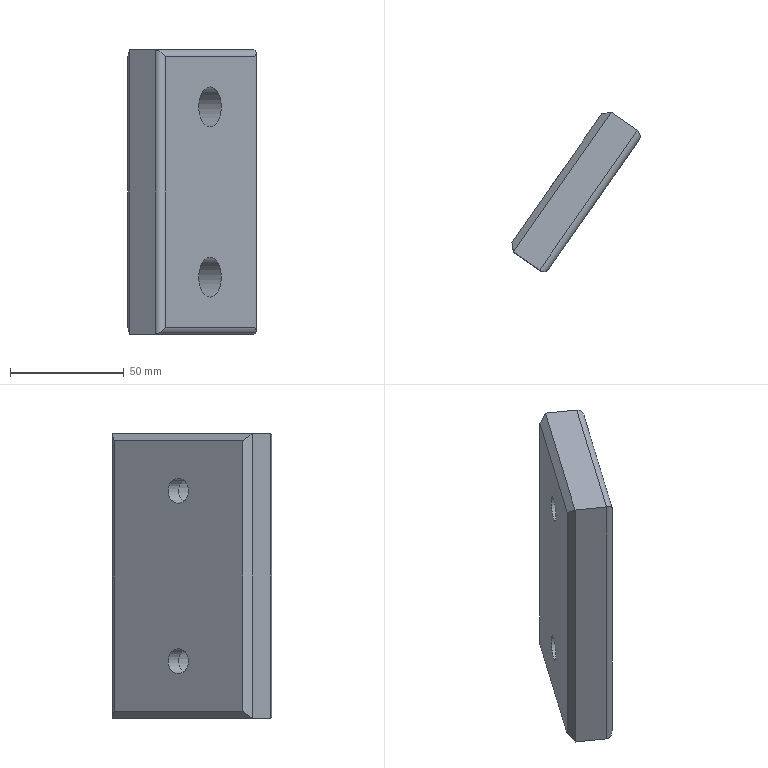Part | NX | features solid 2 | 1 solid | 20 faces | box 56.502 x 70.009 x 125 mm | volume 177681 mm3 | plane 12 | cylinder 8 | commonest cylinder face diameters 6 x4 11 x2 17.5 x2
STEP:
#1=CARTESIAN_POINT('',(279.908,328.94,26.883));
#2=VERTEX_POINT('',#1);
#3=CARTESIAN_POINT('',(291.376,320.91,26.883));
#4=VERTEX_POINT('',#3);
#5=CARTESIAN_POINT('',(277.45,330.66,26.883));
#6=DIRECTION('',(0.8192,-0.5736,0.));
#7=VECTOR('',#6,1000.);
#8=LINE('',#5,#7);
#9=EDGE_CURVE('',#2,#4,#8,.T.);
#10=ORIENTED_EDGE('',*,*,#9,.F.);
#11=CARTESIAN_POINT('',(236.889,267.503,26.883));
#12=VERTEX_POINT('',#11);
#13=CARTESIAN_POINT('',(236.889,267.503,26.883));
#14=DIRECTION('',(-0.5736,-0.8192,0.));
#15=VECTOR('',#14,1000.);
#16=LINE('',#13,#15);
#17=EDGE_CURVE('',#2,#12,#16,.T.);
#18=ORIENTED_EDGE('',*,*,#17,.T.);
#19=CARTESIAN_POINT('',(248.357,259.473,26.883));
#20=VERTEX_POINT('',#19);
#21=CARTESIAN_POINT('',(234.432,269.224,26.883));
#22=DIRECTION('',(0.8192,-0.5736,0.));
#23=VECTOR('',#22,1000.);
#24=LINE('',#21,#23);
#25=EDGE_CURVE('',#12,#20,#24,.T.);
#26=ORIENTED_EDGE('',*,*,#25,.T.);
#27=CARTESIAN_POINT('',(248.357,259.473,26.883));
#28=DIRECTION('',(0.5736,0.8192,0.));
#29=VECTOR('',#28,1000.);
#30=LINE('',#27,#29);
#31=EDGE_CURVE('',#20,#4,#30,.T.);
#32=ORIENTED_EDGE('',*,*,#31,.T.);
#33=EDGE_LOOP('',(#10,#18,#26,#32));
#34=FACE_BOUND('',#33,.T.);
#35=CARTESIAN_POINT('',(234.432,269.224,26.883));
#36=DIRECTION('',(0.,0.,-1.));
#37=DIRECTION('',(0.8192,-0.5736,0.));
#38=AXIS2_PLACEMENT_3D('',#35,#36,#37);
#39=PLANE('',#38);
#40=ADVANCED_FACE('',(#34),#39,.F.);
#41=CARTESIAN_POINT('',(279.908,328.94,-98.117));
#42=VERTEX_POINT('',#41);
#43=CARTESIAN_POINT('',(291.376,320.91,-98.117));
#44=VERTEX_POINT('',#43);
#45=CARTESIAN_POINT('',(277.45,330.66,-98.117));
#46=DIRECTION('',(0.8192,-0.5736,0.));
#47=VECTOR('',#46,1000.);
#48=LINE('',#45,#47);
#49=EDGE_CURVE('',#42,#44,#48,.T.);
#50=ORIENTED_EDGE('',*,*,#49,.F.);
#51=CARTESIAN_POINT('',(279.908,328.94,26.883));
#52=DIRECTION('',(0.,0.,1.));
#53=VECTOR('',#52,1000.);
#54=LINE('',#51,#53);
#55=EDGE_CURVE('',#42,#2,#54,.T.);
#56=ORIENTED_EDGE('',*,*,#55,.T.);
#57=ORIENTED_EDGE('',*,*,#9,.T.);
#58=CARTESIAN_POINT('',(291.376,320.91,26.883));
#59=DIRECTION('',(0.,0.,-1.));
#60=VECTOR('',#59,1000.);
#61=LINE('',#58,#60);
#62=EDGE_CURVE('',#4,#44,#61,.T.);
#63=ORIENTED_EDGE('',*,*,#62,.T.);
#64=EDGE_LOOP('',(#50,#56,#57,#63));
#65=FACE_BOUND('',#64,.T.);
#66=CARTESIAN_POINT('',(277.45,330.66,26.883));
#67=DIRECTION('',(-0.5736,-0.8192,0.));
#68=DIRECTION('',(-0.8192,0.5736,0.));
#69=AXIS2_PLACEMENT_3D('',#66,#67,#68);
#70=PLANE('',#69);
#71=ADVANCED_FACE('',(#65),#70,.F.);
#72=CARTESIAN_POINT('',(236.889,267.503,-98.117));
#73=VERTEX_POINT('',#72);
#74=CARTESIAN_POINT('',(248.357,259.473,-98.117));
#75=VERTEX_POINT('',#74);
#76=CARTESIAN_POINT('',(234.432,269.224,-98.117));
#77=DIRECTION('',(0.8192,-0.5736,0.));
#78=VECTOR('',#77,1000.);
#79=LINE('',#76,#78);
#80=EDGE_CURVE('',#73,#75,#79,.T.);
#81=ORIENTED_EDGE('',*,*,#80,.F.);
#82=CARTESIAN_POINT('',(279.908,328.94,-98.117));
#83=DIRECTION('',(0.5736,0.8192,0.));
#84=VECTOR('',#83,1000.);
#85=LINE('',#82,#84);
#86=EDGE_CURVE('',#73,#42,#85,.T.);
#87=ORIENTED_EDGE('',*,*,#86,.T.);
#88=ORIENTED_EDGE('',*,*,#49,.T.);
#89=CARTESIAN_POINT('',(291.376,320.91,-98.117));
#90=DIRECTION('',(-0.5736,-0.8192,0.));
#91=VECTOR('',#90,1000.);
#92=LINE('',#89,#91);
#93=EDGE_CURVE('',#44,#75,#92,.T.);
#94=ORIENTED_EDGE('',*,*,#93,.T.);
#95=EDGE_LOOP('',(#81,#87,#88,#94));
#96=FACE_BOUND('',#95,.T.);
#97=CARTESIAN_POINT('',(277.45,330.66,-98.117));
#98=DIRECTION('',(0.,0.,1.));
#99=DIRECTION('',(-0.8192,0.5736,0.));
#100=AXIS2_PLACEMENT_3D('',#97,#98,#99);
#101=PLANE('',#100);
#102=ADVANCED_FACE('',(#96),#101,.F.);
#103=ORIENTED_EDGE('',*,*,#25,.F.);
#104=CARTESIAN_POINT('',(236.889,267.503,-173.117));
#105=DIRECTION('',(0.,0.,-1.));
#106=VECTOR('',#105,1000.);
#107=LINE('',#104,#106);
#108=EDGE_CURVE('',#12,#73,#107,.T.);
#109=ORIENTED_EDGE('',*,*,#108,.T.);
#110=ORIENTED_EDGE('',*,*,#80,.T.);
#111=CARTESIAN_POINT('',(248.357,259.473,-173.117));
#112=DIRECTION('',(0.,0.,1.));
#113=VECTOR('',#112,1000.);
#114=LINE('',#111,#113);
#115=EDGE_CURVE('',#75,#20,#114,.T.);
#116=ORIENTED_EDGE('',*,*,#115,.T.);
#117=EDGE_LOOP('',(#103,#109,#110,#116));
#118=FACE_BOUND('',#117,.T.);
#119=CARTESIAN_POINT('',(234.432,269.224,-173.117));
#120=DIRECTION('',(0.5736,0.8192,0.));
#121=DIRECTION('',(0.,0.,-1.));
#122=AXIS2_PLACEMENT_3D('',#119,#120,#121);
#123=PLANE('',#122);
#124=ADVANCED_FACE('',(#118),#123,.F.);
#125=CARTESIAN_POINT('',(275.729,328.203,23.883));
#126=VERTEX_POINT('',#125);
#127=CARTESIAN_POINT('',(275.729,328.203,-95.117));
#128=VERTEX_POINT('',#127);
#129=CARTESIAN_POINT('',(275.729,328.203,-173.117));
#130=DIRECTION('',(0.,0.,-1.));
#131=VECTOR('',#130,1000.);
#132=LINE('',#129,#131);
#133=EDGE_CURVE('',#126,#128,#132,.T.);
#134=ORIENTED_EDGE('',*,*,#133,.T.);
#135=CARTESIAN_POINT('',(236.153,271.681,-95.117));
#136=VERTEX_POINT('',#135);
#137=CARTESIAN_POINT('',(234.432,269.224,-95.117));
#138=DIRECTION('',(-0.5736,-0.8192,0.));
#139=VECTOR('',#138,1000.);
#140=LINE('',#137,#139);
#141=EDGE_CURVE('',#128,#136,#140,.T.);
#142=ORIENTED_EDGE('',*,*,#141,.T.);
#143=CARTESIAN_POINT('',(236.153,271.681,23.883));
#144=VERTEX_POINT('',#143);
#145=CARTESIAN_POINT('',(236.153,271.681,26.883));
#146=DIRECTION('',(0.,0.,1.));
#147=VECTOR('',#146,1000.);
#148=LINE('',#145,#147);
#149=EDGE_CURVE('',#136,#144,#148,.T.);
#150=ORIENTED_EDGE('',*,*,#149,.T.);
#151=CARTESIAN_POINT('',(277.45,330.66,23.883));
#152=DIRECTION('',(0.5736,0.8192,0.));
#153=VECTOR('',#152,1000.);
#154=LINE('',#151,#153);
#155=EDGE_CURVE('',#144,#126,#154,.T.);
#156=ORIENTED_EDGE('',*,*,#155,.T.);
#157=EDGE_LOOP('',(#134,#142,#150,#156));
#158=FACE_BOUND('',#157,.T.);
#159=CARTESIAN_POINT('',(255.941,299.942,-78.617));
#160=VERTEX_POINT('',#159);
#161=CARTESIAN_POINT('',(255.941,299.942,-73.117));
#162=DIRECTION('',(-0.8192,0.5736,0.));
#163=DIRECTION('',(0.,0.,-1.));
#164=AXIS2_PLACEMENT_3D('',#161,#162,#163);
#165=CIRCLE('',#164,5.5);
#166=EDGE_CURVE('',#160,#160,#165,.T.);
#167=ORIENTED_EDGE('',*,*,#166,.F.);
#168=EDGE_LOOP('',(#167));
#169=FACE_BOUND('',#168,.T.);
#170=CARTESIAN_POINT('',(255.941,299.942,-3.617));
#171=VERTEX_POINT('',#170);
#172=CARTESIAN_POINT('',(255.941,299.942,1.883));
#173=DIRECTION('',(-0.8192,0.5736,0.));
#174=DIRECTION('',(0.,0.,-1.));
#175=AXIS2_PLACEMENT_3D('',#172,#173,#174);
#176=CIRCLE('',#175,5.5);
#177=EDGE_CURVE('',#171,#171,#176,.T.);
#178=ORIENTED_EDGE('',*,*,#177,.F.);
#179=EDGE_LOOP('',(#178));
#180=FACE_BOUND('',#179,.T.);
#181=CARTESIAN_POINT('',(277.45,330.66,26.883));
#182=DIRECTION('',(-0.8192,0.5736,0.));
#183=DIRECTION('',(0.,0.,-1.));
#184=AXIS2_PLACEMENT_3D('',#181,#182,#183);
#185=PLANE('',#184);
#186=ADVANCED_FACE('',(#158,#169,#180),#185,.T.);
#187=CARTESIAN_POINT('',(292.112,316.731,23.883));
#188=VERTEX_POINT('',#187);
#189=CARTESIAN_POINT('',(252.536,260.21,23.883));
#190=VERTEX_POINT('',#189);
#191=CARTESIAN_POINT('',(293.833,319.189,23.883));
#192=DIRECTION('',(0.5736,0.8192,0.));
#193=VECTOR('',#192,1000.);
#194=LINE('',#191,#193);
#195=EDGE_CURVE('',#188,#190,#194,.F.);
#196=ORIENTED_EDGE('',*,*,#195,.T.);
#197=CARTESIAN_POINT('',(252.536,260.21,-95.117));
#198=VERTEX_POINT('',#197);
#199=CARTESIAN_POINT('',(252.536,260.21,26.883));
#200=DIRECTION('',(0.,0.,1.));
#201=VECTOR('',#200,1000.);
#202=LINE('',#199,#201);
#203=EDGE_CURVE('',#190,#198,#202,.F.);
#204=ORIENTED_EDGE('',*,*,#203,.T.);
#205=CARTESIAN_POINT('',(292.112,316.731,-95.117));
#206=VERTEX_POINT('',#205);
#207=CARTESIAN_POINT('',(293.833,319.189,-95.117));
#208=DIRECTION('',(-0.5736,-0.8192,0.));
#209=VECTOR('',#208,1000.);
#210=LINE('',#207,#209);
#211=EDGE_CURVE('',#198,#206,#210,.F.);
#212=ORIENTED_EDGE('',*,*,#211,.T.);
#213=CARTESIAN_POINT('',(292.112,316.731,26.883));
#214=DIRECTION('',(0.,0.,-1.));
#215=VECTOR('',#214,1000.);
#216=LINE('',#213,#215);
#217=EDGE_CURVE('',#206,#188,#216,.F.);
#218=ORIENTED_EDGE('',*,*,#217,.T.);
#219=EDGE_LOOP('',(#196,#204,#212,#218));
#220=FACE_BOUND('',#219,.T.);
#221=CARTESIAN_POINT('',(272.324,288.471,-81.867));
#222=VERTEX_POINT('',#221);
#223=CARTESIAN_POINT('',(272.324,288.471,-73.117));
#224=DIRECTION('',(-0.8192,0.5736,0.));
#225=DIRECTION('',(0.,0.,-1.));
#226=AXIS2_PLACEMENT_3D('',#223,#224,#225);
#227=CIRCLE('',#226,8.75);
#228=EDGE_CURVE('',#222,#222,#227,.T.);
#229=ORIENTED_EDGE('',*,*,#228,.T.);
#230=EDGE_LOOP('',(#229));
#231=FACE_BOUND('',#230,.T.);
#232=CARTESIAN_POINT('',(272.324,288.471,-6.867));
#233=VERTEX_POINT('',#232);
#234=CARTESIAN_POINT('',(272.324,288.471,1.883));
#235=DIRECTION('',(-0.8192,0.5736,0.));
#236=DIRECTION('',(0.,0.,-1.));
#237=AXIS2_PLACEMENT_3D('',#234,#235,#236);
#238=CIRCLE('',#237,8.75);
#239=EDGE_CURVE('',#233,#233,#238,.T.);
#240=ORIENTED_EDGE('',*,*,#239,.T.);
#241=EDGE_LOOP('',(#240));
#242=FACE_BOUND('',#241,.T.);
#243=CARTESIAN_POINT('',(293.833,319.189,26.883));
#244=DIRECTION('',(-0.8192,0.5736,0.));
#245=DIRECTION('',(0.,0.,-1.));
#246=AXIS2_PLACEMENT_3D('',#243,#244,#245);
#247=PLANE('',#246);
#248=ADVANCED_FACE('',(#220,#231,#242),#247,.F.);
#249=ORIENTED_EDGE('',*,*,#177,.T.);
#250=EDGE_LOOP('',(#249));
#251=FACE_BOUND('',#250,.T.);
#252=CARTESIAN_POINT('',(262.494,295.354,-3.617));
#253=VERTEX_POINT('',#252);
#254=CARTESIAN_POINT('',(262.494,295.354,1.883));
#255=DIRECTION('',(-0.8192,0.5736,0.));
#256=DIRECTION('',(0.,0.,-1.));
#257=AXIS2_PLACEMENT_3D('',#254,#255,#256);
#258=CIRCLE('',#257,5.5);
#259=EDGE_CURVE('',#253,#253,#258,.T.);
#260=ORIENTED_EDGE('',*,*,#259,.F.);
#261=EDGE_LOOP('',(#260));
#262=FACE_BOUND('',#261,.T.);
#263=CARTESIAN_POINT('',(231.366,317.15,1.883));
#264=DIRECTION('',(-0.8192,0.5736,0.));
#265=DIRECTION('',(0.,0.,-1.));
#266=AXIS2_PLACEMENT_3D('',#263,#264,#265);
#267=CYLINDRICAL_SURFACE('',#266,5.5);
#268=ADVANCED_FACE('',(#251,#262),#267,.F.);
#269=ORIENTED_EDGE('',*,*,#259,.T.);
#270=EDGE_LOOP('',(#269));
#271=FACE_BOUND('',#270,.T.);
#272=CARTESIAN_POINT('',(262.494,295.354,-6.867));
#273=VERTEX_POINT('',#272);
#274=CARTESIAN_POINT('',(262.494,295.354,1.883));
#275=DIRECTION('',(-0.8192,0.5736,0.));
#276=DIRECTION('',(0.,0.,-1.));
#277=AXIS2_PLACEMENT_3D('',#274,#275,#276);
#278=CIRCLE('',#277,8.75);
#279=EDGE_CURVE('',#273,#273,#278,.T.);
#280=ORIENTED_EDGE('',*,*,#279,.F.);
#281=EDGE_LOOP('',(#280));
#282=FACE_BOUND('',#281,.T.);
#283=CARTESIAN_POINT('',(262.494,295.354,1.883));
#284=DIRECTION('',(-0.8192,0.5736,0.));
#285=DIRECTION('',(0.,0.,-1.));
#286=AXIS2_PLACEMENT_3D('',#283,#284,#285);
#287=PLANE('',#286);
#288=ADVANCED_FACE('',(#271,#282),#287,.F.);
#289=ORIENTED_EDGE('',*,*,#279,.T.);
#290=EDGE_LOOP('',(#289));
#291=FACE_BOUND('',#290,.T.);
#292=ORIENTED_EDGE('',*,*,#239,.F.);
#293=EDGE_LOOP('',(#292));
#294=FACE_BOUND('',#293,.T.);
#295=CARTESIAN_POINT('',(272.324,288.471,1.883));
#296=DIRECTION('',(-0.8192,0.5736,0.));
#297=DIRECTION('',(0.,0.,-1.));
#298=AXIS2_PLACEMENT_3D('',#295,#296,#297);
#299=CYLINDRICAL_SURFACE('',#298,8.75);
#300=ADVANCED_FACE('',(#291,#294),#299,.F.);
#301=ORIENTED_EDGE('',*,*,#166,.T.);
#302=EDGE_LOOP('',(#301));
#303=FACE_BOUND('',#302,.T.);
#304=CARTESIAN_POINT('',(262.494,295.354,-78.617));
#305=VERTEX_POINT('',#304);
#306=CARTESIAN_POINT('',(262.494,295.354,-73.117));
#307=DIRECTION('',(-0.8192,0.5736,0.));
#308=DIRECTION('',(0.,0.,-1.));
#309=AXIS2_PLACEMENT_3D('',#306,#307,#308);
#310=CIRCLE('',#309,5.5);
#311=EDGE_CURVE('',#305,#305,#310,.T.);
#312=ORIENTED_EDGE('',*,*,#311,.F.);
#313=EDGE_LOOP('',(#312));
#314=FACE_BOUND('',#313,.T.);
#315=CARTESIAN_POINT('',(231.366,317.15,-73.117));
#316=DIRECTION('',(-0.8192,0.5736,0.));
#317=DIRECTION('',(0.,0.,-1.));
#318=AXIS2_PLACEMENT_3D('',#315,#316,#317);
#319=CYLINDRICAL_SURFACE('',#318,5.5);
#320=ADVANCED_FACE('',(#303,#314),#319,.F.);
#321=ORIENTED_EDGE('',*,*,#311,.T.);
#322=EDGE_LOOP('',(#321));
#323=FACE_BOUND('',#322,.T.);
#324=CARTESIAN_POINT('',(262.494,295.354,-81.867));
#325=VERTEX_POINT('',#324);
#326=CARTESIAN_POINT('',(262.494,295.354,-73.117));
#327=DIRECTION('',(-0.8192,0.5736,0.));
#328=DIRECTION('',(0.,0.,-1.));
#329=AXIS2_PLACEMENT_3D('',#326,#327,#328);
#330=CIRCLE('',#329,8.75);
#331=EDGE_CURVE('',#325,#325,#330,.T.);
#332=ORIENTED_EDGE('',*,*,#331,.F.);
#333=EDGE_LOOP('',(#332));
#334=FACE_BOUND('',#333,.T.);
#335=CARTESIAN_POINT('',(262.494,295.354,-73.117));
#336=DIRECTION('',(-0.8192,0.5736,0.));
#337=DIRECTION('',(0.,0.,-1.));
#338=AXIS2_PLACEMENT_3D('',#335,#336,#337);
#339=PLANE('',#338);
#340=ADVANCED_FACE('',(#323,#334),#339,.F.);
#341=ORIENTED_EDGE('',*,*,#331,.T.);
#342=EDGE_LOOP('',(#341));
#343=FACE_BOUND('',#342,.T.);
#344=ORIENTED_EDGE('',*,*,#228,.F.);
#345=EDGE_LOOP('',(#344));
#346=FACE_BOUND('',#345,.T.);
#347=CARTESIAN_POINT('',(272.324,288.471,-73.117));
#348=DIRECTION('',(-0.8192,0.5736,0.));
#349=DIRECTION('',(0.,0.,-1.));
#350=AXIS2_PLACEMENT_3D('',#347,#348,#349);
#351=CYLINDRICAL_SURFACE('',#350,8.75);
#352=ADVANCED_FACE('',(#343,#346),#351,.F.);
#353=CARTESIAN_POINT('',(289.655,318.452,23.883));
#354=DIRECTION('',(0.4056,0.5792,-0.7071));
#355=DIRECTION('',(0.4056,0.5792,0.7071));
#356=AXIS2_PLACEMENT_3D('',#353,#354,#355);
#357=ELLIPSE('',#356,4.243,3.);
#358=EDGE_CURVE('',#188,#4,#357,.F.);
#359=ORIENTED_EDGE('',*,*,#358,.F.);
#360=ORIENTED_EDGE('',*,*,#217,.F.);
#361=CARTESIAN_POINT('',(289.655,318.452,-95.117));
#362=DIRECTION('',(-0.4056,-0.5792,-0.7071));
#363=DIRECTION('',(0.4056,0.5792,-0.7071));
#364=AXIS2_PLACEMENT_3D('',#361,#362,#363);
#365=ELLIPSE('',#364,4.243,3.);
#366=EDGE_CURVE('',#44,#206,#365,.T.);
#367=ORIENTED_EDGE('',*,*,#366,.F.);
#368=ORIENTED_EDGE('',*,*,#62,.F.);
#369=EDGE_LOOP('',(#359,#360,#367,#368));
#370=FACE_BOUND('',#369,.T.);
#371=CARTESIAN_POINT('',(289.655,318.452,26.883));
#372=DIRECTION('',(0.,0.,-1.));
#373=DIRECTION('',(0.8192,-0.5736,0.));
#374=AXIS2_PLACEMENT_3D('',#371,#372,#373);
#375=CYLINDRICAL_SURFACE('',#374,3.);
#376=ADVANCED_FACE('',(#370),#375,.T.);
#377=ORIENTED_EDGE('',*,*,#366,.T.);
#378=ORIENTED_EDGE('',*,*,#211,.F.);
#379=CARTESIAN_POINT('',(250.078,261.931,-95.117));
#380=DIRECTION('',(-0.4056,-0.5792,0.7071));
#381=DIRECTION('',(-0.4056,-0.5792,-0.7071));
#382=AXIS2_PLACEMENT_3D('',#379,#380,#381);
#383=ELLIPSE('',#382,4.243,3.);
#384=EDGE_CURVE('',#75,#198,#383,.T.);
#385=ORIENTED_EDGE('',*,*,#384,.F.);
#386=ORIENTED_EDGE('',*,*,#93,.F.);
#387=EDGE_LOOP('',(#377,#378,#385,#386));
#388=FACE_BOUND('',#387,.T.);
#389=CARTESIAN_POINT('',(291.376,320.91,-95.117));
#390=DIRECTION('',(-0.5736,-0.8192,0.));
#391=DIRECTION('',(-0.8192,0.5736,0.));
#392=AXIS2_PLACEMENT_3D('',#389,#390,#391);
#393=CYLINDRICAL_SURFACE('',#392,3.);
#394=ADVANCED_FACE('',(#388),#393,.T.);
#395=ORIENTED_EDGE('',*,*,#358,.T.);
#396=ORIENTED_EDGE('',*,*,#31,.F.);
#397=CARTESIAN_POINT('',(250.078,261.931,23.883));
#398=DIRECTION('',(0.4056,0.5792,0.7071));
#399=DIRECTION('',(0.4056,0.5792,-0.7071));
#400=AXIS2_PLACEMENT_3D('',#397,#398,#399);
#401=ELLIPSE('',#400,4.243,3.);
#402=EDGE_CURVE('',#190,#20,#401,.F.);
#403=ORIENTED_EDGE('',*,*,#402,.F.);
#404=ORIENTED_EDGE('',*,*,#195,.F.);
#405=EDGE_LOOP('',(#395,#396,#403,#404));
#406=FACE_BOUND('',#405,.T.);
#407=CARTESIAN_POINT('',(248.357,259.473,23.883));
#408=DIRECTION('',(0.5736,0.8192,0.));
#409=DIRECTION('',(0.8192,-0.5736,0.));
#410=AXIS2_PLACEMENT_3D('',#407,#408,#409);
#411=CYLINDRICAL_SURFACE('',#410,3.);
#412=ADVANCED_FACE('',(#406),#411,.T.);
#413=ORIENTED_EDGE('',*,*,#384,.T.);
#414=ORIENTED_EDGE('',*,*,#203,.F.);
#415=ORIENTED_EDGE('',*,*,#402,.T.);
#416=ORIENTED_EDGE('',*,*,#115,.F.);
#417=EDGE_LOOP('',(#413,#414,#415,#416));
#418=FACE_BOUND('',#417,.T.);
#419=CARTESIAN_POINT('',(250.078,261.931,-173.117));
#420=DIRECTION('',(0.,0.,1.));
#421=DIRECTION('',(0.5736,0.8192,0.));
#422=AXIS2_PLACEMENT_3D('',#419,#420,#421);
#423=CYLINDRICAL_SURFACE('',#422,3.);
#424=ADVANCED_FACE('',(#418),#423,.T.);
#425=CARTESIAN_POINT('',(236.398,270.289,24.883));
#426=DIRECTION('',(-0.1418,0.8041,-0.5774));
#427=VECTOR('',#426,1000.);
#428=LINE('',#425,#427);
#429=EDGE_CURVE('',#12,#144,#428,.T.);
#430=ORIENTED_EDGE('',*,*,#429,.F.);
#431=ORIENTED_EDGE('',*,*,#17,.F.);
#432=CARTESIAN_POINT('',(277.122,328.449,24.883));
#433=DIRECTION('',(-0.8041,-0.1418,-0.5774));
#434=VECTOR('',#433,1000.);
#435=LINE('',#432,#434);
#436=EDGE_CURVE('',#126,#2,#435,.F.);
#437=ORIENTED_EDGE('',*,*,#436,.F.);
#438=ORIENTED_EDGE('',*,*,#155,.F.);
#439=EDGE_LOOP('',(#430,#431,#437,#438));
#440=FACE_BOUND('',#439,.T.);
#441=CARTESIAN_POINT('',(277.45,330.66,23.883));
#442=DIRECTION('',(-0.5792,0.4056,0.7071));
#443=DIRECTION('',(-0.5792,0.4056,-0.7071));
#444=AXIS2_PLACEMENT_3D('',#441,#442,#443);
#445=PLANE('',#444);
#446=ADVANCED_FACE('',(#440),#445,.T.);
#447=ORIENTED_EDGE('',*,*,#436,.T.);
#448=ORIENTED_EDGE('',*,*,#55,.F.);
#449=CARTESIAN_POINT('',(184.274,312.077,-29.451));
#450=DIRECTION('',(-0.8041,-0.1418,0.5774));
#451=VECTOR('',#450,1000.);
#452=LINE('',#449,#451);
#453=EDGE_CURVE('',#128,#42,#452,.F.);
#454=ORIENTED_EDGE('',*,*,#453,.F.);
#455=ORIENTED_EDGE('',*,*,#133,.F.);
#456=EDGE_LOOP('',(#447,#448,#454,#455));
#457=FACE_BOUND('',#456,.T.);
#458=CARTESIAN_POINT('',(275.729,328.203,26.883));
#459=DIRECTION('',(-0.1736,0.9848,0.));
#460=DIRECTION('',(0.9848,0.1736,0.));
#461=AXIS2_PLACEMENT_3D('',#458,#459,#460);
#462=PLANE('',#461);
#463=ADVANCED_FACE('',(#457),#462,.T.);
#464=ORIENTED_EDGE('',*,*,#429,.T.);
#465=ORIENTED_EDGE('',*,*,#149,.F.);
#466=CARTESIAN_POINT('',(220.026,363.137,-29.451));
#467=DIRECTION('',(0.1418,-0.8041,-0.5774));
#468=VECTOR('',#467,1000.);
#469=LINE('',#466,#468);
#470=EDGE_CURVE('',#73,#136,#469,.F.);
#471=ORIENTED_EDGE('',*,*,#470,.F.);
#472=ORIENTED_EDGE('',*,*,#108,.F.);
#473=EDGE_LOOP('',(#464,#465,#471,#472));
#474=FACE_BOUND('',#473,.T.);
#475=CARTESIAN_POINT('',(236.153,271.681,26.883));
#476=DIRECTION('',(-0.9848,-0.1736,0.));
#477=DIRECTION('',(-0.1736,0.9848,0.));
#478=AXIS2_PLACEMENT_3D('',#475,#476,#477);
#479=PLANE('',#478);
#480=ADVANCED_FACE('',(#474),#479,.T.);
#481=ORIENTED_EDGE('',*,*,#453,.T.);
#482=ORIENTED_EDGE('',*,*,#86,.F.);
#483=ORIENTED_EDGE('',*,*,#470,.T.);
#484=ORIENTED_EDGE('',*,*,#141,.F.);
#485=EDGE_LOOP('',(#481,#482,#483,#484));
#486=FACE_BOUND('',#485,.T.);
#487=CARTESIAN_POINT('',(277.45,330.66,-95.117));
#488=DIRECTION('',(-0.5792,0.4056,-0.7071));
#489=DIRECTION('',(0.5792,-0.4056,-0.7071));
#490=AXIS2_PLACEMENT_3D('',#487,#488,#489);
#491=PLANE('',#490);
#492=ADVANCED_FACE('',(#486),#491,.T.);
#493=CLOSED_SHELL('',(#40,#71,#102,#124,#186,#248,#268,#288,#300,#320,#340,#352,#376,#394,#412,#424,#446,#463,#480,#492));
#494=MANIFOLD_SOLID_BREP('',#493);
#495=(LENGTH_UNIT()NAMED_UNIT(*)SI_UNIT(.MILLI.,.METRE.));
#496=UNCERTAINTY_MEASURE_WITH_UNIT(LENGTH_MEASURE(0.00001),#495,'','');
#497=(NAMED_UNIT(*)PLANE_ANGLE_UNIT()SI_UNIT($,.RADIAN.));
#498=(NAMED_UNIT(*)SI_UNIT($,.STERADIAN.)SOLID_ANGLE_UNIT());
#499=(GEOMETRIC_REPRESENTATION_CONTEXT(3)GLOBAL_UNCERTAINTY_ASSIGNED_CONTEXT((#496))GLOBAL_UNIT_ASSIGNED_CONTEXT((#495,#497,#498))REPRESENTATION_CONTEXT('',''));
#500=ADVANCED_BREP_SHAPE_REPRESENTATION('',(#494),#499);